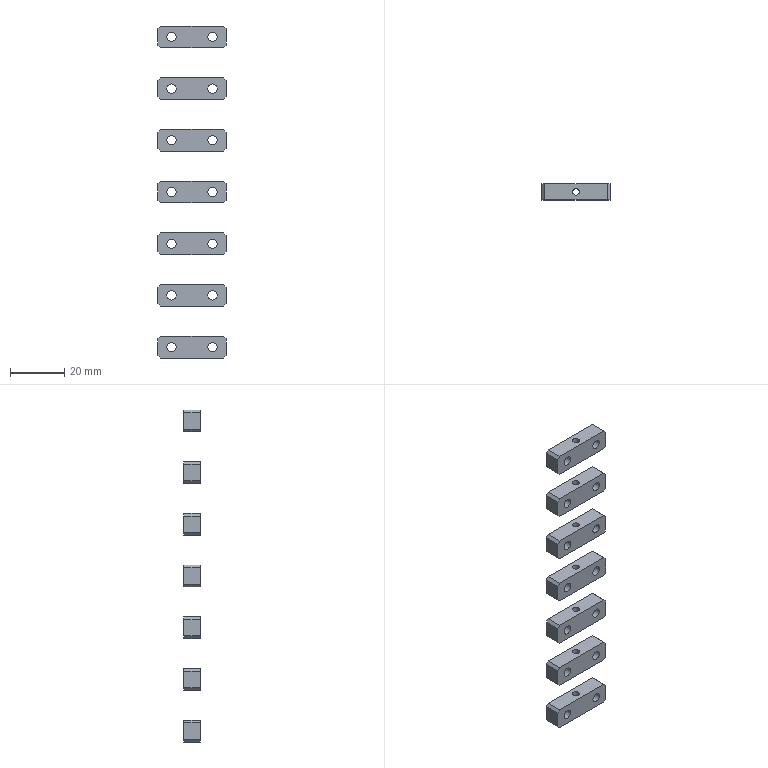CAM job | NX | 3+2 milling, drilling | part box 25 x 6 x 122 mm | stock box 30 x 8 x 127 mm
Tools:
number,name,description,diameter,corner_radius,flute_length,length,flutes
4,D4,平底铣刀-粗,4.0,0.0,25.0,75.0,2
9,D10,平底铣刀-粗,10.0,0.0,35.0,75.0,2
11,D4-J,平底铣刀-精,4.0,0.0,50.0,75.0,2
10,D10-J,平底铣刀-精,10.0,0.0,35.0,75.0,2
1,D80R0.8飞刀,圆鼻刀-粗,80.0,0.8,50.0,75.0,2
2,D6倒角刀,倒角刀,6.0,0.0,3.0,25.0,2
13,ZT3.4,钻头,3.4,0.0,35.0,50.0,2
Operations:
program,operation,operation_type,tool,method,geometry_group,spindle_rpm,surface_speed,feed_per_tooth,feed_cut,feed_plunge,cut_length_mm,path_length_mm,cut_time_min,machine_time_min
A,顶面,FaceMilling,D80R0.8飞刀,侧刃精光-切深K-步距G,W-A,4000.0,1005.31,0.125,1000.0,100.0,216.0,252.0,0.216,0.2196
A,外形粗_2,VolumeBased25DMillingOperation,D10,METHOD,W-A,8000.0,251.327,0.3125,5000.0,80.0,10059.229,10522.662,2.012,2.058
A,沉头孔打点-深0.8,Operation,D6倒角刀,NONE,W-A,8000.0,150.796,0.0312,500.0,90.0,25.2,322.791,0.0504,0.0802
A,沉头孔-钻孔0段,Operation,ZT3.4,NONE,W-A,2800.0,29.908,0.0179,100.0,90.0,140.3,552.992,1.403,1.444
A,铣孔开粗D4_1,CylinderMilling,D4,NONE,W-A,8000.0,100.531,0.075,1200.0,100.0,1149.385,1968.985,0.9578,1.04
A,铣孔精光D4_1,CylinderMilling,D4-J,精光步距切深关,W-A,8000.0,100.531,0.0312,500.0,100.0,218.167,1037.767,0.4363,0.5183
A,仅选体,SurfaceContour,D6倒角刀,METHOD,W-A,8000.0,150.796,0.1875,3000.0,100.0,566.71,943.606,0.1889,0.2266
A,铣倒角_1,PlanarMilling,D6倒角刀,NONE,W-A,8000.0,150.796,0.0312,500.0,100.0,387.585,1135.532,0.7752,0.85
A,外形半精_2,VolumeBased25DMillingOperation,D10-J,METHOD,W-A,8000.0,251.327,0.0625,1000.0,100.0,703.288,1236.89,0.7033,0.7566